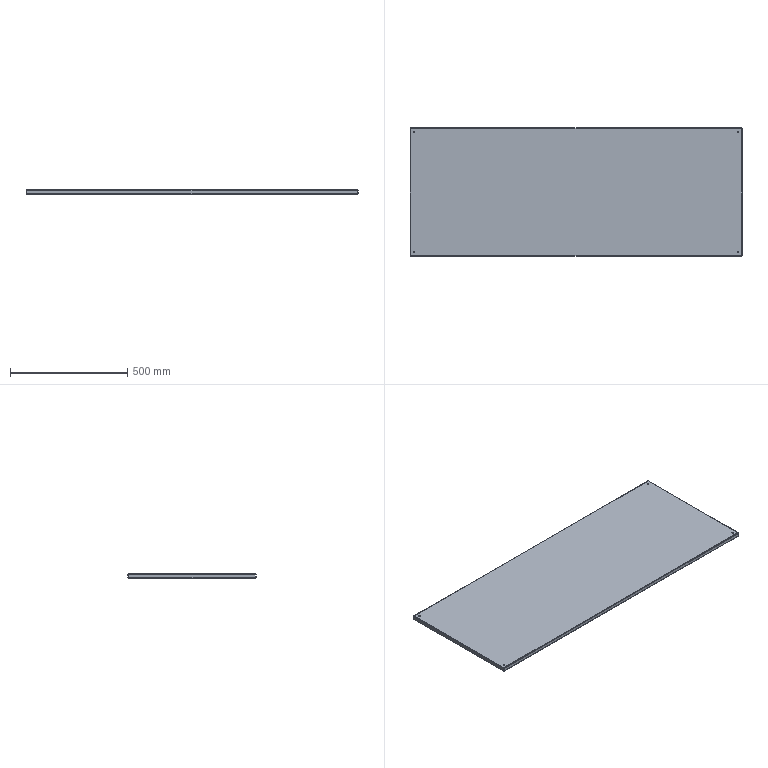Part | STEP file | QA-衬Plate-1 | 1 solid | 78 faces | box 1416 x 546 x 18 mm | volume 1751680 mm3 | plane 38 | cylinder 24 | spline 16 | commonest cylinder face diameters 1.473 x8 5.473 x8 6.5 x8